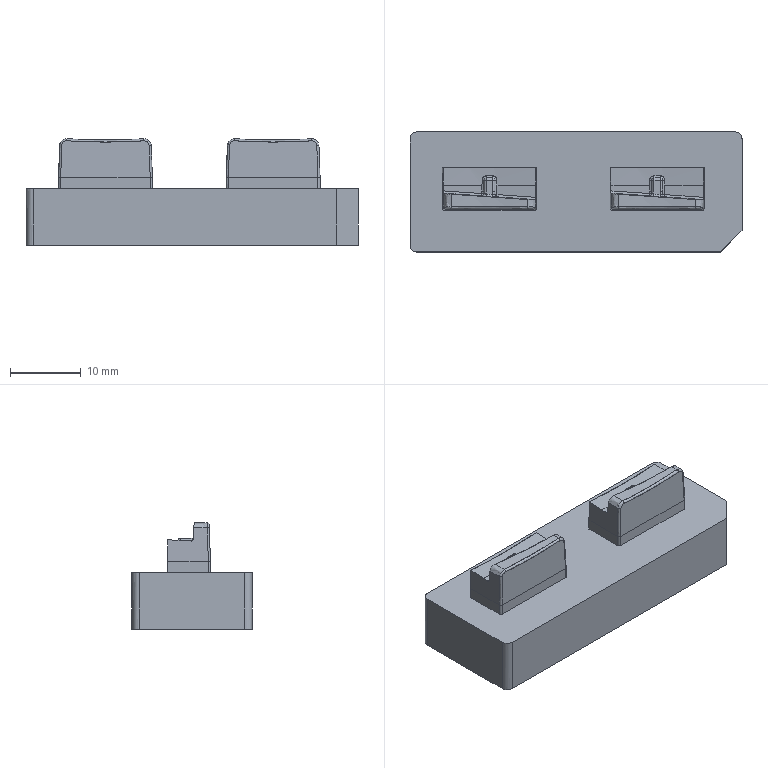NC program | PowerMill | posted with a generic post | part box 47 x 17 x 15.061 mm
Lines 10597 to 11429 of 212044:
N10694 M6
N10695 S8500 M03
N10696 G00 G90 X0.0 Y0.0
N10697 G43 Z9.8009 H3
N10698
N10699 G05 P10000 R8
N10700 X4.4228 Y19.255
N10701 Z-6.06
N10702 G01 Z-7.26 F360.0
N10703 Y13.98 F600.0
N10704 X0.1831 Y6.2919
N10705 G03 X0.4242 Y6.5267 I-0.5673 J0.8235
N10706 G01 X0.5663 Y6.7219
N10707 X0.7103 Y6.9027
N10708 X0.8686 Y7.0836
N10709 X1.1327 Y7.3533
N10710 X1.3024 Y7.5079
N10711 X1.472 Y7.6502
N10712 X1.699 Y7.8229
N10713 X1.9822 Y8.0134
N10714 X2.2654 Y8.1793
N10715 X2.5838 Y8.3395
N10716 X2.8317 Y8.4466
N10717 X3.1149 Y8.5516
N10718 X3.3981 Y8.6389
N10719 X3.6813 Y8.7096
N10720 X3.9644 Y8.7642
N10721 X4.0925 Y8.7836
N10722 X4.5308 Y8.827
N10723 X5.0971 Y8.8362
N10724 X18.1231
N10725 X18.4063 Y8.8293
N10726 X18.6895 Y8.8074
N10727 X18.8833 Y8.7836
N10728 X19.2558 Y8.718
N10729 X19.539 Y8.6495
N10730 X19.8222 Y8.5645
N10731 X20.1054 Y8.462
N10732 X20.3885 Y8.3409
N10733 X20.6399 Y8.2169
N10734 X20.9549 Y8.0373
N10735 X21.2292 Y7.8565
N10736 X21.5212 Y7.6361
N10737 X21.8044 Y7.3897
N10738 X21.9512 Y7.2473
N10739 X22.1072 Y7.0836
N10740 X22.3485 Y6.8002
N10741 X22.5585 Y6.5169
N10742 X22.6539 Y6.3741
N10743 X22.784 Y6.1621
N10744 X22.9012 Y5.9502
N10745 X23.039 Y5.6668
N10746 X23.1569 Y5.3835
N10747 X23.2203 Y5.2095
N10748 X23.3392 Y4.8168
N10749 X23.405 Y4.5335
N10750 X23.4553 Y4.2501
N10751 X23.49 Y3.9668
N10752 X23.5093 Y3.6834
N10753 X23.5137 Y3.1168
N10754 X23.5065 Y-1.9834
N10755 X23.501 Y-2.5501
N10756 X23.4818 Y-2.8334
N10757 X23.4493 Y-3.1168
N10758 X23.4018 Y-3.4001
N10759 X23.3389 Y-3.6834
N10760 X23.2203 Y-4.0946
N10761 X23.1664 Y-4.2501
N10762 X23.055 Y-4.5335
N10763 X22.9258 Y-4.8168
N10764 X22.7977 Y-5.0621
N10765 X22.6061 Y-5.3835
N10766 X22.4123 Y-5.6668
N10767 X22.191 Y-5.9502
N10768 X22.0876 Y-6.0703
N10769 X21.8805 Y-6.2936
N10770 X21.6482 Y-6.5169
N10771 X21.5212 Y-6.6292
N10772 X21.2381 Y-6.8567
N10773 X20.9129 Y-7.0836
N10774 X20.6507 Y-7.2433
N10775 X20.3885 Y-7.3849
N10776 X20.1054 Y-7.5183
N10777 X19.7763 Y-7.6502
N10778 X19.5161 Y-7.7384
N10779 X19.2558 Y-7.8127
N10780 X18.9727 Y-7.8788
N10781 X18.6895 Y-7.9297
N10782 X18.4063 Y-7.9656
N10783 X18.1231 Y-7.9875
N10784 X17.5568 Y-7.9958
N10785 X5.0971 Y-7.9956
N10786 X4.814 Y-7.9854
N10787 X4.5308 Y-7.9615
N10788 X4.2476 Y-7.9237
N10789 X3.9644 Y-7.8708
N10790 X3.6813 Y-7.8022
N10791 X3.3981 Y-7.7189
N10792 X3.1995 Y-7.6502
N10793 X2.8317 Y-7.5014
N10794 X2.5486 Y-7.3653
N10795 X2.2654 Y-7.2083
N10796 X2.0627 Y-7.0836
N10797 X1.8809 Y-6.9608
N10798 X1.699 Y-6.8276
N10799 X1.5132 Y-6.679
N10800 X1.3274 Y-6.5169
N10801 X1.1327 Y-6.3315
N10802 X0.9512 Y-6.1408
N10803 X0.7848 Y-5.9502
N10804 X0.5663 Y-5.6707
N10805 X0.4408 Y-5.4876
N10806 G03 X-1.2095 Y-5.4886 I-0.8248 J-0.5654
N10807 G01 X-1.3314 Y-5.6668
N10808 X-1.553 Y-5.9502
N10809 X-1.699 Y-6.1181
N10810 X-1.8869 Y-6.3175
N10811 X-2.0956 Y-6.5169
N10812 X-2.2654 Y-6.6655
N10813 X-2.5483 Y-6.8884
N10814 X-2.8317 Y-7.0841
N10815 X-3.1149 Y-7.2557
N10816 X-3.3981 Y-7.4062
N10817 X-3.6813 Y-7.5367
N10818 X-3.9644 Y-7.6491
N10819 X-4.2493 Y-7.7452
N10820 X-4.5308 Y-7.8235
N10821 X-4.814 Y-7.8875
N10822 X-5.0971 Y-7.9361
N10823 X-5.3803 Y-7.9697
N10824 X-5.6635 Y-7.9897
N10825 X-6.2298 Y-7.9958
N10826 X-18.6895 Y-7.995
N10827 X-18.9727 Y-7.9824
N10828 X-19.2558 Y-7.9568
N10829 X-19.539 Y-7.9167
N10830 X-19.8222 Y-7.8614
N10831 X-20.1054 Y-7.7906
N10832 X-20.3885 Y-7.705
N10833 X-20.5445 Y-7.6502
N10834 X-20.9549 Y-7.482
N10835 X-21.2381 Y-7.3429
N10836 X-21.5212 Y-7.1829
N10837 X-21.6811 Y-7.0836
N10838 X-21.8843 Y-6.9458
N10839 X-22.0876 Y-6.7947
N10840 X-22.252 Y-6.6612
N10841 X-22.4164 Y-6.5169
N10842 X-22.6539 Y-6.2883
N10843 X-22.8122 Y-6.1192
N10844 X-22.9592 Y-5.9502
N10845 X-23.0948 Y-5.7808
N10846 X-23.2203 Y-5.6115
N10847 X-23.3743 Y-5.3835
N10848 X-23.5447 Y-5.1002
N10849 X-23.694 Y-4.8168
N10850 X-23.7866 Y-4.6181
N10851 X-23.9346 Y-4.2501
N10852 X-24.029 Y-3.9668
N10853 X-24.1071 Y-3.6834
N10854 X-24.1698 Y-3.4001
N10855 X-24.2175 Y-3.1168
N10856 X-24.2498 Y-2.8334
N10857 X-24.2692 Y-2.5501
N10858 X-24.2747 Y-1.9834
N10859 X-24.2819 Y3.1168
N10860 X-24.2775 Y3.6834
N10861 X-24.2579 Y3.9668
N10862 X-24.2236 Y4.2501
N10863 X-24.1734 Y4.5335
N10864 X-24.1074 Y4.8168
N10865 X-24.025 Y5.1002
N10866 X-23.9252 Y5.3835
N10867 X-23.7866 Y5.7117
N10868 X-23.6694 Y5.9502
N10869 X-23.51 Y6.2335
N10870 X-23.3267 Y6.5169
N10871 X-23.2203 Y6.6655
N10872 X-23.0567 Y6.8745
N10873 X-22.8754 Y7.0836
N10874 X-22.6539 Y7.3121
N10875 X-22.4628 Y7.4894
N10876 X-22.2718 Y7.6502
N10877 X-22.0876 Y7.7919
N10878 X-21.8044 Y7.9864
N10879 X-21.5212 Y8.1558
N10880 X-21.4081 Y8.2169
N10881 X-21.1815 Y8.3294
N10882 X-20.9549 Y8.4291
N10883 X-20.6717 Y8.5369
N10884 X-20.3885 Y8.6267
N10885 X-20.1054 Y8.6998
N10886 X-19.8222 Y8.757
N10887 X-19.6516 Y8.7836
N10888 X-19.2558 Y8.8246
N10889 X-18.9727 Y8.8358
N10890 X-5.6635 Y8.8362
N10891 X-5.3803 Y8.8313
N10892 X-5.0971 Y8.8116
N10893 X-4.8607 Y8.7836
N10894 X-4.5308 Y8.7269
N10895 X-4.2476 Y8.6609
N10896 X-3.9644 Y8.5783
N10897 X-3.6813 Y8.4786
N10898 X-3.3981 Y8.3605
N10899 X-3.1041 Y8.2169
N10900 X-2.8317 Y8.0633
N10901 X-2.5486 Y7.8803
N10902 X-2.2405 Y7.6502
N10903 X-1.9698 Y7.4176
N10904 X-1.699 Y7.1508
N10905 X-1.6368 Y7.0836
N10906 X-1.3954 Y6.8002
N10907 X-1.1873 Y6.5197
N10908 G03 X0.1831 Y6.2919 I0.8031 J0.5957
N10909 G00 Z9.8009
N10910 G05 P0
N10911 (---------------)
N10912 ( END TOOLPATH : 精公基准台01-基准面偏置-D10 )
N10913 (---------------)
N10914 ( START TOOLPATH : 精公基准台01-外形侧光-D10 )
N10915 (---------------)
N10916 G00 X0.0 Y0.0 Z10.801
N10917 G05 P10000 R8
N10918 X-1.457 Y-6.0936
N10919 Z-6.03
N10920 G01 Z-7.23 F360.0
N10921 G03 X-2.5561 Y-6.4252 I-0.1493 J-1.4926 F600.0
N10922 G02 X-5.8418 Y-7.625 I-3.3631 J4.1108
N10923 G01 X-18.6227 Y-7.6255
N10924 G02 X-22.6222 Y-5.7748 I0.0298 J5.3111
N10925 G02 X-23.9038 Y-2.3733 I4.0293 J3.4604
N10926 G01 X-23.9122 Y3.4703
N10927 G02 X-18.9859 Y8.4653 I5.01 J-0.0143
N10928 G01 X-12.2313 Y8.4657
N10929 X-5.6585 Y8.466
N10930 G02 X-0.5999 Y3.4685 I0.0478 J-5.0105
N10931 G01 X-0.6084 Y-2.3756
N10932 G02 X-2.5561 Y-6.4252 I-5.3108 J0.0612
N10933 G03 X-3.0989 Y-7.4368 I0.9498 J-1.161
N10934 G01 X-1.5234 Y-6.0503
N10935 G03 X-2.6239 Y-6.3772 I-0.1556 J-1.4919
N10936 G02 X-5.8418 Y-7.545 I-3.2953 J4.0628
N10937 G01 X-18.6207 Y-7.5456
N10938 G02 X-22.5615 Y-5.7226 I0.0278 J5.2312
N10939 G02 X-23.8238 Y-2.3732 I3.9686 J3.4082
N10940 G01 X-23.8322 Y3.4686
N10941 G02 X-18.8033 Y8.386 I4.933 J-0.0147
N10942 G01 X-12.2313
N10943 X-5.6592
N10944 G02 X-0.6799 Y3.4686 I0.0485 J-4.9305
N10945 G01 X-0.6883 Y-2.3732
N10946 G02 X-2.6239 Y-6.3772 I-5.2309 J0.0588
N10947 G03 X-3.1709 Y-7.3866 I0.9449 J-1.165
N10948 G00 Z3.8776
N10949 G01 X22.234 Y-6.1553 F10000.0
N10950 G00 Z-6.03
N10951 G01 Z-7.23 F360.0
N10952 G03 X21.1303 Y-6.4715 I-0.1701 J-1.4903 F600.0
N10953 G02 X17.8905 Y-7.6252 I-3.3057 J4.1571
N10954 G01 X5.1095 Y-7.6255
N10955 G02 X-0.1205 Y-2.9627 I0.0415 J5.3111
N10956 G02 X-0.1599 Y-2.3733 I5.2715 J0.6483
N10957 G01 X-0.1683 Y3.4703
N10958 G02 X0.0185 Y4.8088 I4.8971 J-0.0008
N10959 G02 X4.929 Y8.466 I4.8245 J-1.3527
N10960 G01 X18.0737
N10961 G02 X23.144 Y3.4685 I0.0591 J-5.0108
N10962 G01 X23.1356 Y-2.3756
N10963 G02 X21.1303 Y-6.4715 I-5.3109 J0.0612
N10964 G03 X20.5736 Y-7.4755 I0.9336 J-1.1741
N10965 G01 X22.1677 Y-6.1115
N10966 G03 X21.0627 Y-6.423 I-0.1765 J-1.4896
N10967 G02 X17.8905 Y-7.5452 I-3.238 J4.1086
N10968 G01 X5.1116 Y-7.5455
N10969 G02 X-0.0411 Y-2.953 I0.0394 J5.2311
N10970 G02 X-0.0799 Y-2.3732 I5.1921 J0.6386
N10971 G01 X-0.0883 Y3.4686
N10972 G02 X0.0952 Y4.7864 I4.8167 J0.0009
N10973 G02 X4.929 Y8.386 I4.7478 J-1.3302
N10974 G01 X18.0731
N10975 G02 X23.064 Y3.4686 I0.0597 J-4.9308
N10976 G01 X23.0556 Y-2.3732
N10977 G02 X21.0627 Y-6.423 I-5.2309 J0.0588
N10978 G03 X20.5016 Y-7.4246 I0.9285 J-1.1781
N10979 G00 Z10.801
N10980 G05 P0
N10981 (---------------)
N10982 ( END TOOLPATH : 精公基准台01-外形侧光-D10 )
N10983 (---------------)
N10984 ( START TOOLPATH : 精公基准台01-基准台侧光-D10 )
N10985 (---------------)
N10986 G00 X0.0 Y0.0 Z9.8009
N10987 G05 P10000 R8
N10988 X28.4465 Y-14.8088
N10989 Z-13.96
N10990 G01 Z-15.16 F360.0
N10991 G03 X24.9109 Y-11.2733 I-1.7678 J1.7677 F600.0
N10992 G01 X24.1141 Y-12.0701
N10993 X24.1135 Y-12.0707
N10994 X24.113 Y-12.0712
N10995 X23.9244 Y-12.2523
N10996 X23.9231 Y-12.2535
N10997 X23.9217 Y-12.2548
N10998 X23.7673 Y-12.3899
N10999 X23.766 Y-12.391
N11000 X23.7647 Y-12.392
N11001 X23.603 Y-12.5221
N11002 X23.6011 Y-12.5236
N11003 X23.5992 Y-12.525
N11004 X23.2831 Y-12.7498
N11005 X23.2806 Y-12.7515
N11006 X23.278 Y-12.7531
N11007 X22.9618 Y-12.9436
N11008 X22.9599 Y-12.9447
N11009 X22.958 Y-12.9458
N11010 X22.7937 Y-13.0327
N11011 X22.7924 Y-13.0333
N11012 X22.7912 Y-13.034
N11013 X22.6393 Y-13.1076
N11014 X22.6375 Y-13.1084
N11015 X22.6356 Y-13.1093
N11016 X22.3194 Y-13.243
N11017 X22.3169 Y-13.244
N11018 X22.3144 Y-13.2449
N11019 X21.9991 Y-13.3537
N11020 X21.9965 Y-13.3546
N11021 X21.994 Y-13.3553
N11022 X21.677 Y-13.4417
N11023 X21.6745 Y-13.4424
N11024 X21.672 Y-13.4429
N11025 X21.3558 Y-13.5074
N11026 X21.3533 Y-13.5078
N11027 X21.3507 Y-13.5082
N11028 X21.0346 Y-13.5518
N11029 X21.0321 Y-13.5521
N11030 X21.0295 Y-13.5523
N11031 X20.7134 Y-13.5755
N11032 X20.711 Y-13.5756
N11033 X20.7086 Y-13.5757
N11034 X20.3925 Y-13.58
N11035 X20.3919
N11036 X20.3914
N11037 X-22.2883
N11038 X-22.2884
N11039 X-22.2885
N11040 X-22.6047 Y-13.5789
N11041 X-22.6063
N11042 X-22.6079
N11043 X-22.924 Y-13.5652
N11044 X-22.9262 Y-13.565
N11045 X-22.9283 Y-13.5649
N11046 X-23.2444 Y-13.5342
N11047 X-23.2465 Y-13.534
N11048 X-23.2486 Y-13.5337
N11049 X-23.5648 Y-13.486
N11050 X-23.5669 Y-13.4857
N11051 X-23.569 Y-13.4853
N11052 X-23.8852 Y-13.4201
N11053 X-23.887 Y-13.4197
N11054 X-23.8889 Y-13.4192
N11055 X-24.1362 Y-13.3556
N11056 X-24.1384 Y-13.355
N11057 X-24.1405 Y-13.3544
N11058 X-24.5254 Y-13.2324
N11059 X-24.5278 Y-13.2317
N11060 X-24.53 Y-13.2308
N11061 X-24.8462 Y-13.109
N11062 X-24.8478 Y-13.1084
N11063 X-24.8495 Y-13.1077
N11064 X-25.0153 Y-13.0353
N11065 X-25.0164 Y-13.0348
N11066 X-25.0175 Y-13.0343
N11067 X-25.1678 Y-12.9632
N11068 X-25.1693 Y-12.9624
N11069 X-25.1708 Y-12.9617
N11070 X-25.4869 Y-12.7956
N11071 X-25.4885 Y-12.7948
N11072 X-25.49 Y-12.7939
N11073 X-25.6257 Y-12.715
N11074 X-25.6267 Y-12.7143
N11075 X-25.6278 Y-12.7137
N11076 X-25.8082 Y-12.601
N11077 X-25.8098 Y-12.6
N11078 X-25.8114 Y-12.599
N11079 X-26.1055 Y-12.3955
N11080 X-26.1077 Y-12.3939
N11081 X-26.1098 Y-12.3923
N11082 X-26.4479 Y-12.1238
N11083 X-26.4501 Y-12.1219
N11084 X-26.4523 Y-12.12
N11085 X-26.7684 Y-11.8297
N11086 X-26.7697 Y-11.8284
N11087 X-26.771 Y-11.8272
N11088 X-26.844 Y-11.7538
N11089 X-26.8451 Y-11.7527
N11090 X-26.8462 Y-11.7516
N11091 X-27.0893 Y-11.4878
N11092 X-27.0911 Y-11.4857
N11093 X-27.0929 Y-11.4836
N11094 X-27.3883 Y-11.1152
N11095 X-27.3901 Y-11.1129
N11096 X-27.3918 Y-11.1105
N11097 X-27.6098 Y-10.7944
N11098 X-27.6108 Y-10.7927
N11099 X-27.6119 Y-10.7911
N11100 X-27.7308 Y-10.5991
N11101 X-27.7314 Y-10.598
N11102 X-27.7321 Y-10.5969
N11103 X-27.8036 Y-10.4727
N11104 X-27.8044 Y-10.4713
N11105 X-27.8052 Y-10.4698
N11106 X-27.9703 Y-10.1537
N11107 X-27.9713 Y-10.1516
N11108 X-27.9723 Y-10.1495
N11109 X-28.1144 Y-9.8333
N11110 X-28.1153 Y-9.8312
N11111 X-28.1162 Y-9.8291
N11112 X-28.237 Y-9.5129
N11113 X-28.2378 Y-9.5108
N11114 X-28.2385 Y-9.5087
N11115 X-28.3396 Y-9.1926
N11116 X-28.3402 Y-9.1905
N11117 X-28.3408 Y-9.1884
N11118 X-28.4231 Y-8.8722
N11119 X-28.4236 Y-8.87
N11120 X-28.4241 Y-8.8678
N11121 X-28.4876 Y-8.5517
N11122 X-28.4879 Y-8.5497
N11123 X-28.4883 Y-8.5478
N11124 X-28.5357 Y-8.2317
N11125 X-28.536 Y-8.2294
N11126 X-28.5363 Y-8.2271
N11127 X-28.5653 Y-7.911
N11128 X-28.5655 Y-7.909
N11129 X-28.5656 Y-7.9071
N11130 X-28.5792 Y-7.5909
N11131 Y-7.5892
N11132 Y-7.5875
N11133 Y7.5875
N11134 Y7.5891
N11135 Y7.5907
N11136 X-28.5663 Y7.9069
N11137 X-28.5662 Y7.909
N11138 X-28.5661 Y7.9111
N11139 X-28.5363 Y8.2273
N11140 X-28.536 Y8.2294
N11141 X-28.5358 Y8.2315
N11142 X-28.489 Y8.5476
N11143 X-28.4887 Y8.5498
N11144 X-28.4883 Y8.5519
N11145 X-28.424 Y8.868
N11146 X-28.4236 Y8.8701
N11147 X-28.423 Y8.8722
N11148 X-28.3407 Y9.1884
N11149 X-28.3402 Y9.1905
N11150 X-28.3395 Y9.1926
N11151 X-28.2384 Y9.5087
N11152 X-28.2377 Y9.5108
N11153 X-28.2369 Y9.5129
N11154 X-28.1162 Y9.8291
N11155 X-28.1156 Y9.8306
N11156 X-28.1149 Y9.8322
N11157 X-28.0524 Y9.9774
N11158 X-28.0519 Y9.9785
N11159 X-28.0514 Y9.9796
N11160 X-27.9717 Y10.1505
N11161 X-27.9709 Y10.1521
N11162 X-27.9701 Y10.1537
N11163 X-27.8052 Y10.4698
N11164 X-27.8044 Y10.4713
N11165 X-27.8036 Y10.4727
N11166 X-27.7321 Y10.5969
N11167 X-27.7314 Y10.598
N11168 X-27.7308 Y10.5991
N11169 X-27.6121 Y10.791
N11170 X-27.6111 Y10.7926
N11171 X-27.61 Y10.7942
N11172 X-27.4126 Y11.0822
N11173 X-27.4111 Y11.0844
N11174 X-27.4095 Y11.0865
N11175 X-27.1384 Y11.4307
N11176 X-27.1366 Y11.433
N11177 X-27.1347 Y11.4351
N11178 X-26.8465 Y11.7513
N11179 X-26.8453 Y11.7526
N11180 X-26.844 Y11.7538
N11181 X-26.771 Y11.8272
N11182 X-26.7699 Y11.8283
N11183 X-26.7688 Y11.8293
N11184 X-26.5075 Y12.0721
N11185 X-26.5055 Y12.074
N11186 X-26.5033 Y12.0758
N11187 X-26.1323 Y12.3756
N11188 X-26.13 Y12.3774
N11189 X-26.1276 Y12.3791
N11190 X-25.8115 Y12.5985
N11191 X-25.8099 Y12.5996
N11192 X-25.8083 Y12.6006
N11193 X-25.6279 Y12.7136
N11194 X-25.6268 Y12.7143
N11195 X-25.6257 Y12.715
N11196 X-25.49 Y12.7939
N11197 X-25.4885 Y12.7948
N11198 X-25.487 Y12.7956
N11199 X-25.1708 Y12.9619
N11200 X-25.1693 Y12.9627
N11201 X-25.1677 Y12.9635
N11202 X-25.0174 Y13.0343
N11203 X-25.0164 Y13.0348
N11204 X-25.0153 Y13.0353
N11205 X-24.8494 Y13.1077
N11206 X-24.8478 Y13.1084
N11207 X-24.8462 Y13.109
N11208 X-24.5301 Y13.231
N11209 X-24.528 Y13.2318
N11210 X-24.5259 Y13.2325
N11211 X-24.2097 Y13.3346
N11212 X-24.2076 Y13.3353
N11213 X-24.2055 Y13.3359
N11214 X-23.8894 Y13.4191
N11215 X-23.8872 Y13.4197
N11216 X-23.885 Y13.4201
N11217 X-23.5688 Y13.4846
N11218 X-23.5669 Y13.485
N11219 X-23.5649 Y13.4853
N11220 X-23.2488 Y13.5337
N11221 X-23.2465 Y13.534
N11222 X-23.2443 Y13.5342
N11223 X-22.9281 Y13.5642
N11224 X-22.9262 Y13.5644
N11225 X-22.9242 Y13.5645
N11226 X-22.608 Y13.5788
N11227 X-22.6064 Y13.5789
N11228 X-22.6047
N11229 X-22.2885 Y13.58
N11230 X-22.2884
N11231 X-22.2883
N11232 X0.0
N11233 X22.2883
N11234 X22.2884
N11235 X22.2885
N11236 X22.6047 Y13.5789
N11237 X22.6063
N11238 X22.6079 Y13.5788
N11239 X22.924 Y13.5652
N11240 X22.9262 Y13.565
N11241 X22.9283 Y13.5649
N11242 X23.2444 Y13.5342
N11243 X23.2465 Y13.534
N11244 X23.2486 Y13.5337
N11245 X23.5648 Y13.486
N11246 X23.5669 Y13.4857
N11247 X23.569 Y13.4853
N11248 X23.8852 Y13.4201
N11249 X23.887 Y13.4197
N11250 X23.8889 Y13.4192
N11251 X24.1362 Y13.3556
N11252 X24.1384 Y13.355
N11253 X24.1405 Y13.3544
N11254 X24.5254 Y13.2324
N11255 X24.5278 Y13.2317
N11256 X24.53 Y13.2308
N11257 X24.8462 Y13.109
N11258 X24.8478 Y13.1084
N11259 X24.8495 Y13.1077
N11260 X25.0153 Y13.0353
N11261 X25.0164 Y13.0348
N11262 X25.0175 Y13.0343
N11263 X25.1678 Y12.9632
N11264 X25.1693 Y12.9624
N11265 X25.1708 Y12.9617
N11266 X25.4869 Y12.7956
N11267 X25.4885 Y12.7948
N11268 X25.49 Y12.7939
N11269 X25.6257 Y12.715
N11270 X25.6267 Y12.7143
N11271 X25.6278 Y12.7137
N11272 X25.8082 Y12.601
N11273 X25.8098 Y12.6
N11274 X25.8114 Y12.599
N11275 X26.1055 Y12.3955
N11276 X26.1077 Y12.3939
N11277 X26.1098 Y12.3923
N11278 X26.4479 Y12.1238
N11279 X26.4501 Y12.1219
N11280 X26.4523 Y12.12
N11281 X26.7684 Y11.8297
N11282 X26.7697 Y11.8284
N11283 X26.771 Y11.8272
N11284 X26.844 Y11.7538
N11285 X26.8451 Y11.7527
N11286 X26.8462 Y11.7516
N11287 X27.0893 Y11.4878
N11288 X27.0911 Y11.4857
N11289 X27.0929 Y11.4836
N11290 X27.3883 Y11.1152
N11291 X27.3901 Y11.1129
N11292 X27.3918 Y11.1105
N11293 X27.6098 Y10.7944
N11294 X27.6108 Y10.7927
N11295 X27.6119 Y10.7911
N11296 X27.7308 Y10.5991
N11297 X27.7314 Y10.598
N11298 X27.7321 Y10.5969
N11299 X27.8036 Y10.4727
N11300 X27.8044 Y10.4713
N11301 X27.8052 Y10.4698
N11302 X27.9703 Y10.1537
N11303 X27.9713 Y10.1516
N11304 X27.9723 Y10.1495
N11305 X28.1144 Y9.8333
N11306 X28.1153 Y9.8312
N11307 X28.1162 Y9.8291
N11308 X28.237 Y9.5129
N11309 X28.2378 Y9.5108
N11310 X28.2385 Y9.5087
N11311 X28.3396 Y9.1926
N11312 X28.3402 Y9.1905
N11313 X28.3408 Y9.1884
N11314 X28.4231 Y8.8722
N11315 X28.4236 Y8.87
N11316 X28.4241 Y8.8678
N11317 X28.4876 Y8.5517
N11318 X28.4879 Y8.5497
N11319 X28.4883 Y8.5478
N11320 X28.5357 Y8.2317
N11321 X28.536 Y8.2294
N11322 X28.5363 Y8.2271
N11323 X28.5653 Y7.911
N11324 X28.5655 Y7.909
N11325 X28.5656 Y7.9071
N11326 X28.5792 Y7.5909
N11327 Y7.5892
N11328 Y7.5875
N11329 X28.58 Y-5.3745
N11330 Y-5.3749
N11331 Y-5.3754
N11332 X28.5764 Y-5.6915
N11333 X28.5763 Y-5.6939
N11334 X28.5762 Y-5.6962
N11335 X28.5541 Y-6.0123
N11336 X28.5539 Y-6.0149
N11337 X28.5536 Y-6.0174
N11338 X28.5111 Y-6.3336
N11339 X28.5107 Y-6.3361
N11340 X28.5103 Y-6.3386
N11341 X28.447 Y-6.6548
N11342 X28.4465 Y-6.6571
N11343 X28.4459 Y-6.6595
N11344 X28.3724 Y-6.9374
N11345 X28.3717 Y-6.9399
N11346 X28.3709 Y-6.9424
N11347 X28.2515 Y-7.2969
N11348 X28.2506 Y-7.2996
N11349 X28.2495 Y-7.3022
N11350 X28.1172 Y-7.6184
N11351 X28.1164 Y-7.6202
N11352 X28.1156 Y-7.622
N11353 X28.0511 Y-7.757
N11354 X28.0505 Y-7.7583
N11355 X28.0498 Y-7.7595
N11356 X27.9553 Y-7.9407
N11357 X27.9542 Y-7.9427
N11358 X27.953 Y-7.9447
N11359 X27.7643 Y-8.2608
N11360 X27.7627 Y-8.2634
N11361 X27.761 Y-8.2659
N11362 X27.5382 Y-8.582
N11363 X27.5368 Y-8.5839
N11364 X27.5354 Y-8.5858
N11365 X27.4092 Y-8.7442
N11366 X27.4081 Y-8.7454
N11367 X27.4071 Y-8.7467
N11368 X27.2704 Y-8.9045
N11369 X27.2692 Y-8.9059
N11370 X27.2679 Y-8.9072
N11371 X27.0884 Y-9.0958
N11372 X27.0877 Y-9.0965
N11373 X27.087 Y-9.0972
N11374 X24.9109 Y-11.2733
N11375 G03 X28.4465 Y-14.8088 I1.7678 J-1.7678
N11376 G01 X28.3953 Y-14.7469
N11377 G03 X24.8597 Y-11.2113 I-1.7678 J1.7678
N11378 G01 X24.0575 Y-12.0135
N11379 X23.869 Y-12.1946
N11380 X23.7146 Y-12.3297
N11381 X23.5529 Y-12.4598
N11382 X23.2367 Y-12.6846
N11383 X22.9206 Y-12.875
N11384 X22.7563 Y-12.962
N11385 X22.6044 Y-13.0356
N11386 X22.2883 Y-13.1693
N11387 X21.973 Y-13.2781
N11388 X21.656 Y-13.3645
N11389 X21.3398 Y-13.429
N11390 X21.0237 Y-13.4725
N11391 X20.7075 Y-13.4957
N11392 X20.3914 Y-13.5
N11393 X-22.2883
N11394 X-22.6044 Y-13.4989
N11395 X-22.9206 Y-13.4852
N11396 X-23.2367 Y-13.4546
N11397 X-23.5529 Y-13.4069
N11398 X-23.869 Y-13.3417
N11399 X-24.1163 Y-13.2781
N11400 X-24.5013 Y-13.1562
N11401 X-24.8174 Y-13.0344
N11402 X-24.9832 Y-12.962
N11403 X-25.1336 Y-12.8909
N11404 X-25.4497 Y-12.7248
N11405 X-25.5854 Y-12.6458
N11406 X-25.7659 Y-12.5332
N11407 X-26.06 Y-12.3297
N11408 X-26.3982 Y-12.0611
N11409 X-26.7143 Y-11.7707
N11410 X-26.7873 Y-11.6974
N11411 X-27.0305 Y-11.4335
N11412 X-27.3259 Y-11.0651
N11413 X-27.5439 Y-10.749
N11414 X-27.6627 Y-10.557
N11415 X-27.7343 Y-10.4328
N11416 X-27.8993 Y-10.1167
N11417 X-28.0415 Y-9.8005
N11418 X-28.1623 Y-9.4844
N11419 X-28.2634 Y-9.1682
N11420 X-28.3457 Y-8.8521
N11421 X-28.4091 Y-8.5359
N11422 X-28.4566 Y-8.2198
N11423 X-28.4857 Y-7.9036
N11424 X-28.4992 Y-7.5875
N11425 X-28.5 Y-7.2714
N11426 Y7.2714
N11427 X-28.4992 Y7.5875
N11428 X-28.4864 Y7.9036
N11429 X-28.4566 Y8.2198
N11430 X-28.4099 Y8.5359
N11431 X-28.3456 Y8.8521
N11432 X-28.2633 Y9.1682
N11433 X-28.1622 Y9.4844
N11434 X-28.0415 Y9.8005
N11435 X-27.9789 Y9.9458
N11436 X-27.8992 Y10.1167
N11437 X-27.7343 Y10.4328
N11438 X-27.6627 Y10.557
N11439 X-27.544 Y10.749
N11440 X-27.3466 Y11.037
N11441 X-27.0756 Y11.3812
N11442 X-26.7873 Y11.6974
N11443 X-26.7143 Y11.7707
N11444 X-26.4531 Y12.0135
N11445 X-26.082 Y12.3133
N11446 X-25.7659 Y12.5328
N11447 X-25.5854 Y12.6458
N11448 X-25.4497 Y12.7248
N11449 X-25.1336 Y12.8911
N11450 X-24.9833 Y12.962
N11451 X-24.8174 Y13.0344
N11452 X-24.5013 Y13.1564
N11453 X-24.1851 Y13.2585
N11454 X-23.869 Y13.3417
N11455 X-23.5529 Y13.4063
N11456 X-23.2367 Y13.4546
N11457 X-22.9206 Y13.4846
N11458 X-22.6044 Y13.4989
N11459 X-22.2883 Y13.5
N11460 X0.0
N11461 X22.2883
N11462 X22.6044 Y13.4989
N11463 X22.9206 Y13.4852
N11464 X23.2367 Y13.4546
N11465 X23.5529 Y13.4069
N11466 X23.869 Y13.3417
N11467 X24.1163 Y13.2781
N11468 X24.5013 Y13.1562
N11469 X24.8174 Y13.0344
N11470 X24.9832 Y12.962
N11471 X25.1336 Y12.8909
N11472 X25.4497 Y12.7248
N11473 X25.5854 Y12.6458
N11474 X25.7659 Y12.5332
N11475 X26.06 Y12.3297
N11476 X26.3982 Y12.0611
N11477 X26.7143 Y11.7707
N11478 X26.7873 Y11.6974
N11479 X27.0305 Y11.4335
N11480 X27.3259 Y11.0651
N11481 X27.5439 Y10.749
N11482 X27.6627 Y10.557
N11483 X27.7343 Y10.4328
N11484 X27.8993 Y10.1167
N11485 X28.0415 Y9.8005
N11486 X28.1623 Y9.4844
N11487 X28.2634 Y9.1682
N11488 X28.3457 Y8.8521
N11489 X28.4091 Y8.5359
N11490 X28.4566 Y8.2198
N11491 X28.4857 Y7.9036
N11492 X28.4992 Y7.5875
N11493 X28.5 Y7.2714
N11494 Y-5.3745
N11495 X28.4964 Y-5.6906
N11496 X28.4743 Y-6.0068
N11497 X28.4318 Y-6.3229
N11498 X28.3685 Y-6.6391
N11499 X28.295 Y-6.9169
N11500 X28.1757 Y-7.2714
N11501 X28.0434 Y-7.5875
N11502 X27.9789 Y-7.7225
N11503 X27.8844 Y-7.9036
N11504 X27.6956 Y-8.2198
N11505 X27.4728 Y-8.5359
N11506 X27.3466 Y-8.6943
N11507 X27.2099 Y-8.8521
N11508 X27.0305 Y-9.0406
N11509 X24.8597 Y-11.2113
N11510 G03 X28.3953 Y-14.7469 I1.7678 J-1.7678
N11511 G00 Z9.8009
N11512 G05 P0
N11513 (---------------)
N11514 ( END TOOLPATH : 精公基准台01-基准台侧光-D10 )
N11515 (---------------)
N11516
N11517 M05
N11518 G53 Z0.0
N11519 (---------------)
N11520 ( START TOOLPATH : 精公精光01-浅滩和陡峭-R1 )
N11521 (---------------)
N11522 ( TOOL NO.    :4 )
N11523 ( TOOL TYPE   : BALLNOSED)
N11524 ( TOOL ID     : R1_1_1)
N11525 ( TOOL DIA    : 2.0 LENGTH 61.84)
N11526 T4